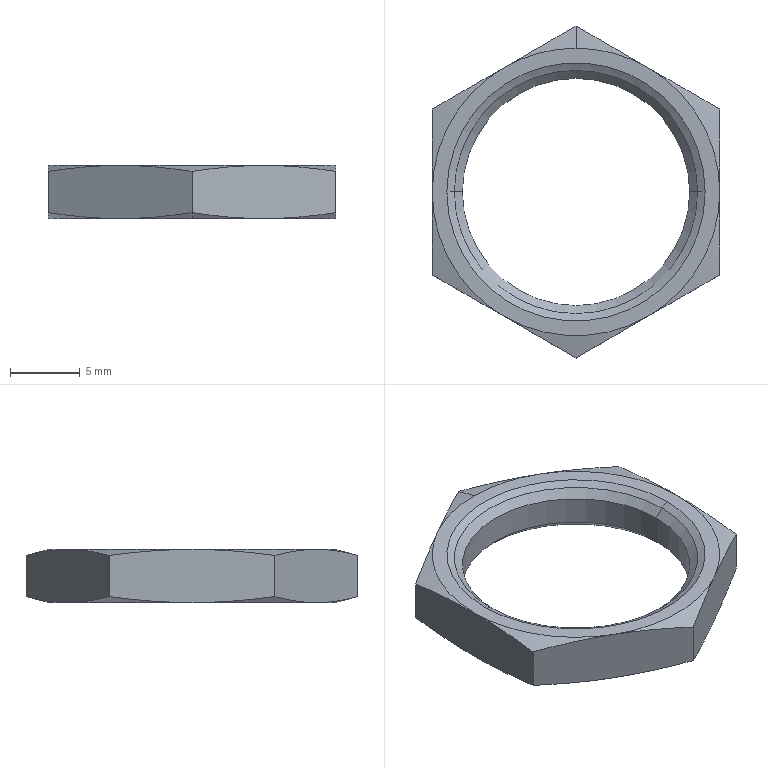Part | SolidWorks | features BaseBody 1 | 1 solid | 32 faces | box 20.638 x 23.83 x 3.81 mm | volume 553.998 mm3 | cone 22 | plane 8 | cylinder 2 | commonest cylinder face diameters 16.317 x2
STEP:
#1=CARTESIAN_POINT('',(8.158,0.,-0.8871));
#2=VERTEX_POINT('',#1);
#3=CARTESIAN_POINT('',(-8.158,0.,-0.8871));
#4=VERTEX_POINT('',#3);
#5=CARTESIAN_POINT('',(0.,0.,-0.8871));
#6=DIRECTION('',(0.,0.,-1.));
#7=DIRECTION('',(-1.,0.,0.));
#8=AXIS2_PLACEMENT_3D('',#5,#6,#7);
#9=CIRCLE('',#8,8.158);
#10=EDGE_CURVE('',#2,#4,#9,.T.);
#11=ORIENTED_EDGE('',*,*,#10,.F.);
#12=CARTESIAN_POINT('',(8.158,0.,-2.923));
#13=VERTEX_POINT('',#12);
#14=CARTESIAN_POINT('',(8.158,0.,-3.81));
#15=DIRECTION('',(0.,0.,-1.));
#16=VECTOR('',#15,1000.);
#17=LINE('',#14,#16);
#18=EDGE_CURVE('',#2,#13,#17,.T.);
#19=ORIENTED_EDGE('',*,*,#18,.T.);
#20=CARTESIAN_POINT('',(-8.158,0.,-2.923));
#21=VERTEX_POINT('',#20);
#22=CARTESIAN_POINT('',(0.,0.,-2.923));
#23=DIRECTION('',(0.,0.,1.));
#24=DIRECTION('',(-1.,0.,0.));
#25=AXIS2_PLACEMENT_3D('',#22,#23,#24);
#26=CIRCLE('',#25,8.158);
#27=EDGE_CURVE('',#21,#13,#26,.T.);
#28=ORIENTED_EDGE('',*,*,#27,.F.);
#29=CARTESIAN_POINT('',(-8.158,0.,-3.81));
#30=DIRECTION('',(0.,0.,-1.));
#31=VECTOR('',#30,1000.);
#32=LINE('',#29,#31);
#33=EDGE_CURVE('',#4,#21,#32,.T.);
#34=ORIENTED_EDGE('',*,*,#33,.F.);
#35=EDGE_LOOP('',(#11,#19,#28,#34));
#36=FACE_OUTER_BOUND('',#35,.T.);
#37=CARTESIAN_POINT('',(0.,0.,-3.81));
#38=DIRECTION('',(0.,0.,-1.));
#39=DIRECTION('',(-1.,0.,0.));
#40=AXIS2_PLACEMENT_3D('',#37,#38,#39);
#41=CYLINDRICAL_SURFACE('',#40,8.158);
#42=ADVANCED_FACE('',(#36),#41,.F.);
#43=ORIENTED_EDGE('',*,*,#10,.T.);
#44=CARTESIAN_POINT('',(-8.738,0.,-0.308));
#45=VERTEX_POINT('',#44);
#46=CARTESIAN_POINT('',(-8.738,0.,-0.308));
#47=DIRECTION('',(-0.7071,0.,0.7071));
#48=VECTOR('',#47,1000.);
#49=LINE('',#46,#48);
#50=EDGE_CURVE('',#4,#45,#49,.T.);
#51=ORIENTED_EDGE('',*,*,#50,.T.);
#52=CARTESIAN_POINT('',(8.738,0.,-0.308));
#53=VERTEX_POINT('',#52);
#54=CARTESIAN_POINT('',(0.,0.,-0.308));
#55=DIRECTION('',(0.,0.,-1.));
#56=DIRECTION('',(1.,0.,0.));
#57=AXIS2_PLACEMENT_3D('',#54,#55,#56);
#58=CIRCLE('',#57,8.738);
#59=EDGE_CURVE('',#53,#45,#58,.T.);
#60=ORIENTED_EDGE('',*,*,#59,.F.);
#61=CARTESIAN_POINT('',(8.738,0.,-0.308));
#62=DIRECTION('',(0.7071,0.,0.7071));
#63=VECTOR('',#62,1000.);
#64=LINE('',#61,#63);
#65=EDGE_CURVE('',#2,#53,#64,.T.);
#66=ORIENTED_EDGE('',*,*,#65,.F.);
#67=EDGE_LOOP('',(#43,#51,#60,#66));
#68=FACE_OUTER_BOUND('',#67,.T.);
#69=CARTESIAN_POINT('',(0.,0.,-0.308));
#70=DIRECTION('',(0.,0.,1.));
#71=DIRECTION('',(1.,0.,0.));
#72=AXIS2_PLACEMENT_3D('',#69,#70,#71);
#73=CONICAL_SURFACE('',#72,8.738,0.7854);
#74=ADVANCED_FACE('',(#68),#73,.F.);
#75=ORIENTED_EDGE('',*,*,#27,.T.);
#76=CARTESIAN_POINT('',(8.738,0.,-3.502));
#77=VERTEX_POINT('',#76);
#78=CARTESIAN_POINT('',(8.738,0.,-3.502));
#79=DIRECTION('',(0.7071,0.,-0.7071));
#80=VECTOR('',#79,1000.);
#81=LINE('',#78,#80);
#82=EDGE_CURVE('',#13,#77,#81,.T.);
#83=ORIENTED_EDGE('',*,*,#82,.T.);
#84=CARTESIAN_POINT('',(0.,-8.738,-3.502));
#85=VERTEX_POINT('',#84);
#86=CARTESIAN_POINT('',(0.,0.,-3.502));
#87=DIRECTION('',(0.,0.,1.));
#88=DIRECTION('',(-1.,0.,0.));
#89=AXIS2_PLACEMENT_3D('',#86,#87,#88);
#90=CIRCLE('',#89,8.738);
#91=EDGE_CURVE('',#85,#77,#90,.T.);
#92=ORIENTED_EDGE('',*,*,#91,.F.);
#93=CARTESIAN_POINT('',(-8.738,0.,-3.502));
#94=VERTEX_POINT('',#93);
#95=CARTESIAN_POINT('',(0.,0.,-3.502));
#96=DIRECTION('',(0.,0.,1.));
#97=DIRECTION('',(-1.,0.,0.));
#98=AXIS2_PLACEMENT_3D('',#95,#96,#97);
#99=CIRCLE('',#98,8.738);
#100=EDGE_CURVE('',#94,#85,#99,.T.);
#101=ORIENTED_EDGE('',*,*,#100,.F.);
#102=CARTESIAN_POINT('',(-8.738,0.,-3.502));
#103=DIRECTION('',(-0.7071,0.,-0.7071));
#104=VECTOR('',#103,1000.);
#105=LINE('',#102,#104);
#106=EDGE_CURVE('',#21,#94,#105,.T.);
#107=ORIENTED_EDGE('',*,*,#106,.F.);
#108=EDGE_LOOP('',(#75,#83,#92,#101,#107));
#109=FACE_OUTER_BOUND('',#108,.T.);
#110=CARTESIAN_POINT('',(0.,0.,-3.502));
#111=DIRECTION('',(0.,0.,-1.));
#112=DIRECTION('',(-1.,0.,0.));
#113=AXIS2_PLACEMENT_3D('',#110,#111,#112);
#114=CONICAL_SURFACE('',#113,8.738,0.7854);
#115=ADVANCED_FACE('',(#109),#114,.F.);
#116=ORIENTED_EDGE('',*,*,#59,.T.);
#117=CARTESIAN_POINT('',(-9.271,0.,0.));
#118=VERTEX_POINT('',#117);
#119=CARTESIAN_POINT('',(-9.271,0.,0.));
#120=DIRECTION('',(-0.866,0.,0.5));
#121=VECTOR('',#120,1000.);
#122=LINE('',#119,#121);
#123=EDGE_CURVE('',#45,#118,#122,.T.);
#124=ORIENTED_EDGE('',*,*,#123,.T.);
#125=CARTESIAN_POINT('',(9.271,0.,0.));
#126=VERTEX_POINT('',#125);
#127=CARTESIAN_POINT('',(0.,0.,0.));
#128=DIRECTION('',(0.,0.,-1.));
#129=DIRECTION('',(1.,0.,0.));
#130=AXIS2_PLACEMENT_3D('',#127,#128,#129);
#131=CIRCLE('',#130,9.271);
#132=EDGE_CURVE('',#126,#118,#131,.T.);
#133=ORIENTED_EDGE('',*,*,#132,.F.);
#134=CARTESIAN_POINT('',(9.271,0.,0.));
#135=DIRECTION('',(0.866,0.,0.5));
#136=VECTOR('',#135,1000.);
#137=LINE('',#134,#136);
#138=EDGE_CURVE('',#53,#126,#137,.T.);
#139=ORIENTED_EDGE('',*,*,#138,.F.);
#140=EDGE_LOOP('',(#116,#124,#133,#139));
#141=FACE_OUTER_BOUND('',#140,.T.);
#142=CARTESIAN_POINT('',(0.,0.,0.));
#143=DIRECTION('',(0.,0.,1.));
#144=DIRECTION('',(1.,0.,0.));
#145=AXIS2_PLACEMENT_3D('',#142,#143,#144);
#146=CONICAL_SURFACE('',#145,9.271,1.047);
#147=ADVANCED_FACE('',(#141),#146,.F.);
#148=CARTESIAN_POINT('',(0.,8.738,-3.502));
#149=VERTEX_POINT('',#148);
#150=CARTESIAN_POINT('',(0.,0.,-3.502));
#151=DIRECTION('',(0.,0.,1.));
#152=DIRECTION('',(-1.,0.,0.));
#153=AXIS2_PLACEMENT_3D('',#150,#151,#152);
#154=CIRCLE('',#153,8.738);
#155=EDGE_CURVE('',#149,#94,#154,.T.);
#156=ORIENTED_EDGE('',*,*,#155,.T.);
#157=ORIENTED_EDGE('',*,*,#100,.T.);
#158=CARTESIAN_POINT('',(0.,-9.271,-3.81));
#159=VERTEX_POINT('',#158);
#160=CARTESIAN_POINT('',(0.,-9.271,-3.81));
#161=DIRECTION('',(0.,-0.866,-0.5));
#162=VECTOR('',#161,1000.);
#163=LINE('',#160,#162);
#164=EDGE_CURVE('',#85,#159,#163,.T.);
#165=ORIENTED_EDGE('',*,*,#164,.T.);
#166=CARTESIAN_POINT('',(0.,9.271,-3.81));
#167=VERTEX_POINT('',#166);
#168=CARTESIAN_POINT('',(0.,0.,-3.81));
#169=DIRECTION('',(0.,0.,1.));
#170=DIRECTION('',(0.,1.,0.));
#171=AXIS2_PLACEMENT_3D('',#168,#169,#170);
#172=CIRCLE('',#171,9.271);
#173=EDGE_CURVE('',#167,#159,#172,.T.);
#174=ORIENTED_EDGE('',*,*,#173,.F.);
#175=CARTESIAN_POINT('',(0.,9.271,-3.81));
#176=DIRECTION('',(0.,0.866,-0.5));
#177=VECTOR('',#176,1000.);
#178=LINE('',#175,#177);
#179=EDGE_CURVE('',#149,#167,#178,.T.);
#180=ORIENTED_EDGE('',*,*,#179,.F.);
#181=EDGE_LOOP('',(#156,#157,#165,#174,#180));
#182=FACE_OUTER_BOUND('',#181,.T.);
#183=CARTESIAN_POINT('',(0.,0.,-3.81));
#184=DIRECTION('',(0.,0.,-1.));
#185=DIRECTION('',(0.,1.,0.));
#186=AXIS2_PLACEMENT_3D('',#183,#184,#185);
#187=CONICAL_SURFACE('',#186,9.271,1.047);
#188=ADVANCED_FACE('',(#182),#187,.F.);
#189=CARTESIAN_POINT('',(-5.159,8.936,0.));
#190=VERTEX_POINT('',#189);
#191=CARTESIAN_POINT('',(0.,10.319,0.));
#192=VERTEX_POINT('',#191);
#193=CARTESIAN_POINT('',(0.,0.,0.));
#194=DIRECTION('',(0.,0.,-1.));
#195=DIRECTION('',(0.,1.,0.));
#196=AXIS2_PLACEMENT_3D('',#193,#194,#195);
#197=CIRCLE('',#196,10.319);
#198=EDGE_CURVE('',#190,#192,#197,.T.);
#199=ORIENTED_EDGE('',*,*,#198,.T.);
#200=CARTESIAN_POINT('',(0.000000011,11.915,-0.4277));
#201=VERTEX_POINT('',#200);
#202=CARTESIAN_POINT('',(0.,11.925,-0.4303));
#203=DIRECTION('',(0.,0.9659,-0.2588));
#204=VECTOR('',#203,1000.);
#205=LINE('',#202,#204);
#206=EDGE_CURVE('',#192,#201,#205,.T.);
#207=ORIENTED_EDGE('',*,*,#206,.T.);
#208=CARTESIAN_POINT('',(0.000000011,11.915,-0.4277));
#209=CARTESIAN_POINT('',(-0.8561,11.421,-0.2953));
#210=CARTESIAN_POINT('',(-1.714,10.926,-0.1874));
#211=CARTESIAN_POINT('',(-3.433,9.933,-0.0395));
#212=CARTESIAN_POINT('',(-4.295,9.435,0.));
#213=CARTESIAN_POINT('',(-5.159,8.936,0.));
#214=B_SPLINE_CURVE_WITH_KNOTS('',3,(#208,#209,#210,#211,#212,#213),.UNSPECIFIED.,.F.,.F.,(4,2,4),(0.,0.002986,0.005973),.UNSPECIFIED.);
#215=EDGE_CURVE('',#201,#190,#214,.T.);
#216=ORIENTED_EDGE('',*,*,#215,.T.);
#217=EDGE_LOOP('',(#199,#207,#216));
#218=FACE_OUTER_BOUND('',#217,.T.);
#219=CARTESIAN_POINT('',(0.,0.,-0.4303));
#220=DIRECTION('',(0.,0.,-1.));
#221=DIRECTION('',(0.,1.,0.));
#222=AXIS2_PLACEMENT_3D('',#219,#220,#221);
#223=CONICAL_SURFACE('',#222,11.925,1.309);
#224=ADVANCED_FACE('',(#218),#223,.T.);
#225=CARTESIAN_POINT('',(-5.159,-8.936,-3.81));
#226=VERTEX_POINT('',#225);
#227=CARTESIAN_POINT('',(0.,-10.319,-3.81));
#228=VERTEX_POINT('',#227);
#229=CARTESIAN_POINT('',(0.,0.,-3.81));
#230=DIRECTION('',(0.,0.,1.));
#231=DIRECTION('',(0.,-1.,0.));
#232=AXIS2_PLACEMENT_3D('',#229,#230,#231);
#233=CIRCLE('',#232,10.319);
#234=EDGE_CURVE('',#226,#228,#233,.T.);
#235=ORIENTED_EDGE('',*,*,#234,.T.);
#236=CARTESIAN_POINT('',(0.000000011,-11.915,-3.382));
#237=VERTEX_POINT('',#236);
#238=CARTESIAN_POINT('',(0.,-11.925,-3.38));
#239=DIRECTION('',(0.,-0.9659,0.2588));
#240=VECTOR('',#239,1000.);
#241=LINE('',#238,#240);
#242=EDGE_CURVE('',#228,#237,#241,.T.);
#243=ORIENTED_EDGE('',*,*,#242,.T.);
#244=CARTESIAN_POINT('',(0.000000011,-11.915,-3.382));
#245=CARTESIAN_POINT('',(-0.8561,-11.421,-3.515));
#246=CARTESIAN_POINT('',(-1.714,-10.926,-3.623));
#247=CARTESIAN_POINT('',(-3.433,-9.933,-3.771));
#248=CARTESIAN_POINT('',(-4.295,-9.435,-3.81));
#249=CARTESIAN_POINT('',(-5.159,-8.936,-3.81));
#250=B_SPLINE_CURVE_WITH_KNOTS('',3,(#244,#245,#246,#247,#248,#249),.UNSPECIFIED.,.F.,.F.,(4,2,4),(0.,0.002986,0.005973),.UNSPECIFIED.);
#251=EDGE_CURVE('',#237,#226,#250,.T.);
#252=ORIENTED_EDGE('',*,*,#251,.T.);
#253=EDGE_LOOP('',(#235,#243,#252));
#254=FACE_OUTER_BOUND('',#253,.T.);
#255=CARTESIAN_POINT('',(0.,0.,-3.38));
#256=DIRECTION('',(0.,0.,1.));
#257=DIRECTION('',(0.,-1.,0.));
#258=AXIS2_PLACEMENT_3D('',#255,#256,#257);
#259=CONICAL_SURFACE('',#258,11.925,1.309);
#260=ADVANCED_FACE('',(#254),#259,.T.);
#261=ORIENTED_EDGE('',*,*,#18,.F.);
#262=CARTESIAN_POINT('',(0.,0.,-0.8871));
#263=DIRECTION('',(0.,0.,-1.));
#264=DIRECTION('',(-1.,0.,0.));
#265=AXIS2_PLACEMENT_3D('',#262,#263,#264);
#266=CIRCLE('',#265,8.158);
#267=EDGE_CURVE('',#4,#2,#266,.T.);
#268=ORIENTED_EDGE('',*,*,#267,.F.);
#269=ORIENTED_EDGE('',*,*,#33,.T.);
#270=CARTESIAN_POINT('',(0.,0.,-2.923));
#271=DIRECTION('',(0.,0.,1.));
#272=DIRECTION('',(-1.,0.,0.));
#273=AXIS2_PLACEMENT_3D('',#270,#271,#272);
#274=CIRCLE('',#273,8.158);
#275=EDGE_CURVE('',#13,#21,#274,.T.);
#276=ORIENTED_EDGE('',*,*,#275,.F.);
#277=EDGE_LOOP('',(#261,#268,#269,#276));
#278=FACE_OUTER_BOUND('',#277,.T.);
#279=CARTESIAN_POINT('',(0.,0.,-3.81));
#280=DIRECTION('',(0.,0.,-1.));
#281=DIRECTION('',(-1.,0.,0.));
#282=AXIS2_PLACEMENT_3D('',#279,#280,#281);
#283=CYLINDRICAL_SURFACE('',#282,8.158);
#284=ADVANCED_FACE('',(#278),#283,.F.);
#285=ORIENTED_EDGE('',*,*,#50,.F.);
#286=ORIENTED_EDGE('',*,*,#267,.T.);
#287=ORIENTED_EDGE('',*,*,#65,.T.);
#288=CARTESIAN_POINT('',(0.,0.,-0.308));
#289=DIRECTION('',(0.,0.,-1.));
#290=DIRECTION('',(1.,0.,0.));
#291=AXIS2_PLACEMENT_3D('',#288,#289,#290);
#292=CIRCLE('',#291,8.738);
#293=EDGE_CURVE('',#45,#53,#292,.T.);
#294=ORIENTED_EDGE('',*,*,#293,.F.);
#295=EDGE_LOOP('',(#285,#286,#287,#294));
#296=FACE_OUTER_BOUND('',#295,.T.);
#297=CARTESIAN_POINT('',(0.,0.,-0.308));
#298=DIRECTION('',(0.,0.,1.));
#299=DIRECTION('',(1.,0.,0.));
#300=AXIS2_PLACEMENT_3D('',#297,#298,#299);
#301=CONICAL_SURFACE('',#300,8.738,0.7854);
#302=ADVANCED_FACE('',(#296),#301,.F.);
#303=ORIENTED_EDGE('',*,*,#82,.F.);
#304=ORIENTED_EDGE('',*,*,#275,.T.);
#305=ORIENTED_EDGE('',*,*,#106,.T.);
#306=ORIENTED_EDGE('',*,*,#155,.F.);
#307=CARTESIAN_POINT('',(0.,0.,-3.502));
#308=DIRECTION('',(0.,0.,1.));
#309=DIRECTION('',(-1.,0.,0.));
#310=AXIS2_PLACEMENT_3D('',#307,#308,#309);
#311=CIRCLE('',#310,8.738);
#312=EDGE_CURVE('',#77,#149,#311,.T.);
#313=ORIENTED_EDGE('',*,*,#312,.F.);
#314=EDGE_LOOP('',(#303,#304,#305,#306,#313));
#315=FACE_OUTER_BOUND('',#314,.T.);
#316=CARTESIAN_POINT('',(0.,0.,-3.502));
#317=DIRECTION('',(0.,0.,-1.));
#318=DIRECTION('',(-1.,0.,0.));
#319=AXIS2_PLACEMENT_3D('',#316,#317,#318);
#320=CONICAL_SURFACE('',#319,8.738,0.7854);
#321=ADVANCED_FACE('',(#315),#320,.F.);
#322=ORIENTED_EDGE('',*,*,#123,.F.);
#323=ORIENTED_EDGE('',*,*,#293,.T.);
#324=ORIENTED_EDGE('',*,*,#138,.T.);
#325=CARTESIAN_POINT('',(0.,0.,0.));
#326=DIRECTION('',(0.,0.,-1.));
#327=DIRECTION('',(1.,0.,0.));
#328=AXIS2_PLACEMENT_3D('',#325,#326,#327);
#329=CIRCLE('',#328,9.271);
#330=EDGE_CURVE('',#118,#126,#329,.T.);
#331=ORIENTED_EDGE('',*,*,#330,.F.);
#332=EDGE_LOOP('',(#322,#323,#324,#331));
#333=FACE_OUTER_BOUND('',#332,.T.);
#334=CARTESIAN_POINT('',(0.,0.,0.));
#335=DIRECTION('',(0.,0.,1.));
#336=DIRECTION('',(1.,0.,0.));
#337=AXIS2_PLACEMENT_3D('',#334,#335,#336);
#338=CONICAL_SURFACE('',#337,9.271,1.047);
#339=ADVANCED_FACE('',(#333),#338,.F.);
#340=ORIENTED_EDGE('',*,*,#164,.F.);
#341=ORIENTED_EDGE('',*,*,#91,.T.);
#342=ORIENTED_EDGE('',*,*,#312,.T.);
#343=ORIENTED_EDGE('',*,*,#179,.T.);
#344=CARTESIAN_POINT('',(0.,0.,-3.81));
#345=DIRECTION('',(0.,0.,1.));
#346=DIRECTION('',(0.,1.,0.));
#347=AXIS2_PLACEMENT_3D('',#344,#345,#346);
#348=CIRCLE('',#347,9.271);
#349=EDGE_CURVE('',#159,#167,#348,.T.);
#350=ORIENTED_EDGE('',*,*,#349,.F.);
#351=EDGE_LOOP('',(#340,#341,#342,#343,#350));
#352=FACE_OUTER_BOUND('',#351,.T.);
#353=CARTESIAN_POINT('',(0.,0.,-3.81));
#354=DIRECTION('',(0.,0.,-1.));
#355=DIRECTION('',(0.,1.,0.));
#356=AXIS2_PLACEMENT_3D('',#353,#354,#355);
#357=CONICAL_SURFACE('',#356,9.271,1.047);
#358=ADVANCED_FACE('',(#352),#357,.F.);
#359=ORIENTED_EDGE('',*,*,#132,.T.);
#360=ORIENTED_EDGE('',*,*,#330,.T.);
#361=EDGE_LOOP('',(#359,#360));
#362=FACE_BOUND('',#361,.T.);
#363=CARTESIAN_POINT('',(-10.319,0.,0.));
#364=VERTEX_POINT('',#363);
#365=CARTESIAN_POINT('',(0.,0.,0.));
#366=DIRECTION('',(0.,0.,-1.));
#367=DIRECTION('',(-1.,0.,0.));
#368=AXIS2_PLACEMENT_3D('',#365,#366,#367);
#369=CIRCLE('',#368,10.319);
#370=EDGE_CURVE('',#364,#190,#369,.T.);
#371=ORIENTED_EDGE('',*,*,#370,.F.);
#372=CARTESIAN_POINT('',(-5.159,-8.936,0.));
#373=VERTEX_POINT('',#372);
#374=CARTESIAN_POINT('',(0.,0.,0.));
#375=DIRECTION('',(0.,0.,-1.));
#376=DIRECTION('',(-1.,0.,0.));
#377=AXIS2_PLACEMENT_3D('',#374,#375,#376);
#378=CIRCLE('',#377,10.319);
#379=EDGE_CURVE('',#373,#364,#378,.T.);
#380=ORIENTED_EDGE('',*,*,#379,.F.);
#381=CARTESIAN_POINT('',(5.159,-8.936,0.));
#382=VERTEX_POINT('',#381);
#383=CARTESIAN_POINT('',(0.,0.,0.));
#384=DIRECTION('',(0.,0.,-1.));
#385=DIRECTION('',(0.,1.,0.));
#386=AXIS2_PLACEMENT_3D('',#383,#384,#385);
#387=CIRCLE('',#386,10.319);
#388=EDGE_CURVE('',#382,#373,#387,.T.);
#389=ORIENTED_EDGE('',*,*,#388,.F.);
#390=CARTESIAN_POINT('',(10.319,0.,0.));
#391=VERTEX_POINT('',#390);
#392=CARTESIAN_POINT('',(0.,0.,0.));
#393=DIRECTION('',(0.,0.,-1.));
#394=DIRECTION('',(-1.,0.,0.));
#395=AXIS2_PLACEMENT_3D('',#392,#393,#394);
#396=CIRCLE('',#395,10.319);
#397=EDGE_CURVE('',#391,#382,#396,.T.);
#398=ORIENTED_EDGE('',*,*,#397,.F.);
#399=CARTESIAN_POINT('',(5.159,8.936,0.));
#400=VERTEX_POINT('',#399);
#401=CARTESIAN_POINT('',(0.,0.,0.));
#402=DIRECTION('',(0.,0.,-1.));
#403=DIRECTION('',(-1.,0.,0.));
#404=AXIS2_PLACEMENT_3D('',#401,#402,#403);
#405=CIRCLE('',#404,10.319);
#406=EDGE_CURVE('',#400,#391,#405,.T.);
#407=ORIENTED_EDGE('',*,*,#406,.F.);
#408=CARTESIAN_POINT('',(0.,0.,0.));
#409=DIRECTION('',(0.,0.,-1.));
#410=DIRECTION('',(0.,1.,0.));
#411=AXIS2_PLACEMENT_3D('',#408,#409,#410);
#412=CIRCLE('',#411,10.319);
#413=EDGE_CURVE('',#192,#400,#412,.T.);
#414=ORIENTED_EDGE('',*,*,#413,.F.);
#415=ORIENTED_EDGE('',*,*,#198,.F.);
#416=EDGE_LOOP('',(#371,#380,#389,#398,#407,#414,#415));
#417=FACE_OUTER_BOUND('',#416,.T.);
#418=CARTESIAN_POINT('',(0.,0.,0.));
#419=DIRECTION('',(0.,0.,-1.));
#420=DIRECTION('',(-1.,0.,0.));
#421=AXIS2_PLACEMENT_3D('',#418,#419,#420);
#422=PLANE('',#421);
#423=ADVANCED_FACE('',(#362,#417),#422,.F.);
#424=CARTESIAN_POINT('',(5.159,8.936,-3.81));
#425=VERTEX_POINT('',#424);
#426=CARTESIAN_POINT('',(-5.159,8.936,-3.81));
#427=VERTEX_POINT('',#426);
#428=CARTESIAN_POINT('',(0.,0.,-3.81));
#429=DIRECTION('',(0.,0.,1.));
#430=DIRECTION('',(0.,-1.,0.));
#431=AXIS2_PLACEMENT_3D('',#428,#429,#430);
#432=CIRCLE('',#431,10.319);
#433=EDGE_CURVE('',#425,#427,#432,.T.);
#434=ORIENTED_EDGE('',*,*,#433,.F.);
#435=CARTESIAN_POINT('',(10.319,0.,-3.81));
#436=VERTEX_POINT('',#435);
#437=CARTESIAN_POINT('',(0.,0.,-3.81));
#438=DIRECTION('',(0.,0.,1.));
#439=DIRECTION('',(1.,0.,0.));
#440=AXIS2_PLACEMENT_3D('',#437,#438,#439);
#441=CIRCLE('',#440,10.319);
#442=EDGE_CURVE('',#436,#425,#441,.T.);
#443=ORIENTED_EDGE('',*,*,#442,.F.);
#444=CARTESIAN_POINT('',(5.159,-8.936,-3.81));
#445=VERTEX_POINT('',#444);
#446=CARTESIAN_POINT('',(0.,0.,-3.81));
#447=DIRECTION('',(0.,0.,1.));
#448=DIRECTION('',(1.,0.,0.));
#449=AXIS2_PLACEMENT_3D('',#446,#447,#448);
#450=CIRCLE('',#449,10.319);
#451=EDGE_CURVE('',#445,#436,#450,.T.);
#452=ORIENTED_EDGE('',*,*,#451,.F.);
#453=CARTESIAN_POINT('',(0.,0.,-3.81));
#454=DIRECTION('',(0.,0.,1.));
#455=DIRECTION('',(0.,-1.,0.));
#456=AXIS2_PLACEMENT_3D('',#453,#454,#455);
#457=CIRCLE('',#456,10.319);
#458=EDGE_CURVE('',#228,#445,#457,.T.);
#459=ORIENTED_EDGE('',*,*,#458,.F.);
#460=ORIENTED_EDGE('',*,*,#234,.F.);
#461=CARTESIAN_POINT('',(-10.319,0.,-3.81));
#462=VERTEX_POINT('',#461);
#463=CARTESIAN_POINT('',(0.,0.,-3.81));
#464=DIRECTION('',(0.,0.,1.));
#465=DIRECTION('',(1.,0.,0.));
#466=AXIS2_PLACEMENT_3D('',#463,#464,#465);
#467=CIRCLE('',#466,10.319);
#468=EDGE_CURVE('',#462,#226,#467,.T.);
#469=ORIENTED_EDGE('',*,*,#468,.F.);
#470=CARTESIAN_POINT('',(0.,0.,-3.81));
#471=DIRECTION('',(0.,0.,1.));
#472=DIRECTION('',(1.,0.,0.));
#473=AXIS2_PLACEMENT_3D('',#470,#471,#472);
#474=CIRCLE('',#473,10.319);
#475=EDGE_CURVE('',#427,#462,#474,.T.);
#476=ORIENTED_EDGE('',*,*,#475,.F.);
#477=EDGE_LOOP('',(#434,#443,#452,#459,#460,#469,#476));
#478=FACE_OUTER_BOUND('',#477,.T.);
#479=ORIENTED_EDGE('',*,*,#173,.T.);
#480=ORIENTED_EDGE('',*,*,#349,.T.);
#481=EDGE_LOOP('',(#479,#480));
#482=FACE_BOUND('',#481,.T.);
#483=CARTESIAN_POINT('',(0.,10.319,-3.81));
#484=DIRECTION('',(0.,0.,1.));
#485=DIRECTION('',(1.,0.,0.));
#486=AXIS2_PLACEMENT_3D('',#483,#484,#485);
#487=PLANE('',#486);
#488=ADVANCED_FACE('',(#478,#482),#487,.F.);
#489=ORIENTED_EDGE('',*,*,#206,.F.);
#490=ORIENTED_EDGE('',*,*,#413,.T.);
#491=CARTESIAN_POINT('',(5.159,8.936,0.));
#492=CARTESIAN_POINT('',(4.295,9.435,0.));
#493=CARTESIAN_POINT('',(3.433,9.933,-0.0395));
#494=CARTESIAN_POINT('',(1.714,10.926,-0.1874));
#495=CARTESIAN_POINT('',(0.8561,11.421,-0.2953));
#496=CARTESIAN_POINT('',(0.000000011,11.915,-0.4277));
#497=B_SPLINE_CURVE_WITH_KNOTS('',3,(#491,#492,#493,#494,#495,#496),.UNSPECIFIED.,.F.,.F.,(4,2,4),(0.,0.002986,0.005973),.UNSPECIFIED.);
#498=EDGE_CURVE('',#400,#201,#497,.T.);
#499=ORIENTED_EDGE('',*,*,#498,.T.);
#500=EDGE_LOOP('',(#489,#490,#499));
#501=FACE_OUTER_BOUND('',#500,.T.);
#502=CARTESIAN_POINT('',(0.,0.,-0.4303));
#503=DIRECTION('',(0.,0.,-1.));
#504=DIRECTION('',(0.,1.,0.));
#505=AXIS2_PLACEMENT_3D('',#502,#503,#504);
#506=CONICAL_SURFACE('',#505,11.925,1.309);
#507=ADVANCED_FACE('',(#501),#506,.T.);
#508=ORIENTED_EDGE('',*,*,#370,.T.);
#509=CARTESIAN_POINT('',(-10.319,5.958,-0.4277));
#510=VERTEX_POINT('',#509);
#511=CARTESIAN_POINT('',(-5.159,8.936,0.));
#512=CARTESIAN_POINT('',(-6.024,8.437,0.));
#513=CARTESIAN_POINT('',(-6.886,7.94,-0.0395));
#514=CARTESIAN_POINT('',(-8.605,6.947,-0.1874));
#515=CARTESIAN_POINT('',(-9.463,6.452,-0.2953));
#516=CARTESIAN_POINT('',(-10.319,5.958,-0.4277));
#517=B_SPLINE_CURVE_WITH_KNOTS('',3,(#511,#512,#513,#514,#515,#516),.UNSPECIFIED.,.F.,.F.,(4,2,4),(0.,0.002986,0.005973),.UNSPECIFIED.);
#518=EDGE_CURVE('',#190,#510,#517,.T.);
#519=ORIENTED_EDGE('',*,*,#518,.T.);
#520=CARTESIAN_POINT('',(-10.319,5.958,-0.4277));
#521=CARTESIAN_POINT('',(-10.319,4.969,-0.2953));
#522=CARTESIAN_POINT('',(-10.319,3.979,-0.1874));
#523=CARTESIAN_POINT('',(-10.319,1.993,-0.0395));
#524=CARTESIAN_POINT('',(-10.319,0.998,0.));
#525=CARTESIAN_POINT('',(-10.319,0.,0.));
#526=B_SPLINE_CURVE_WITH_KNOTS('',3,(#520,#521,#522,#523,#524,#525),.UNSPECIFIED.,.F.,.F.,(4,2,4),(0.,0.002986,0.005973),.UNSPECIFIED.);
#527=EDGE_CURVE('',#510,#364,#526,.T.);
#528=ORIENTED_EDGE('',*,*,#527,.T.);
#529=EDGE_LOOP('',(#508,#519,#528));
#530=FACE_OUTER_BOUND('',#529,.T.);
#531=CARTESIAN_POINT('',(0.,0.,-0.4303));
#532=DIRECTION('',(0.,0.,-1.));
#533=DIRECTION('',(-1.,0.,0.));
#534=AXIS2_PLACEMENT_3D('',#531,#532,#533);
#535=CONICAL_SURFACE('',#534,11.925,1.309);
#536=ADVANCED_FACE('',(#530),#535,.T.);
#537=CARTESIAN_POINT('',(-10.319,-5.958,-0.4277));
#538=VERTEX_POINT('',#537);
#539=CARTESIAN_POINT('',(-10.319,-5.958,-0.4277));
#540=CARTESIAN_POINT('',(-9.463,-6.452,-0.2953));
#541=CARTESIAN_POINT('',(-8.605,-6.947,-0.1874));
#542=CARTESIAN_POINT('',(-6.886,-7.94,-0.0395));
#543=CARTESIAN_POINT('',(-6.024,-8.437,0.));
#544=CARTESIAN_POINT('',(-5.159,-8.936,0.));
#545=B_SPLINE_CURVE_WITH_KNOTS('',3,(#539,#540,#541,#542,#543,#544),.UNSPECIFIED.,.F.,.F.,(4,2,4),(0.,0.002986,0.005973),.UNSPECIFIED.);
#546=EDGE_CURVE('',#538,#373,#545,.T.);
#547=ORIENTED_EDGE('',*,*,#546,.T.);
#548=ORIENTED_EDGE('',*,*,#379,.T.);
#549=CARTESIAN_POINT('',(-10.319,0.,0.));
#550=CARTESIAN_POINT('',(-10.319,-0.998,0.));
#551=CARTESIAN_POINT('',(-10.319,-1.993,-0.0395));
#552=CARTESIAN_POINT('',(-10.319,-3.979,-0.1874));
#553=CARTESIAN_POINT('',(-10.319,-4.969,-0.2953));
#554=CARTESIAN_POINT('',(-10.319,-5.958,-0.4277));
#555=B_SPLINE_CURVE_WITH_KNOTS('',3,(#549,#550,#551,#552,#553,#554),.UNSPECIFIED.,.F.,.F.,(4,2,4),(0.,0.002986,0.005973),.UNSPECIFIED.);
#556=EDGE_CURVE('',#364,#538,#555,.T.);
#557=ORIENTED_EDGE('',*,*,#556,.T.);
#558=EDGE_LOOP('',(#547,#548,#557));
#559=FACE_OUTER_BOUND('',#558,.T.);
#560=CARTESIAN_POINT('',(0.,0.,-0.4303));
#561=DIRECTION('',(0.,0.,-1.));
#562=DIRECTION('',(-1.,0.,0.));
#563=AXIS2_PLACEMENT_3D('',#560,#561,#562);
#564=CONICAL_SURFACE('',#563,11.925,1.309);
#565=ADVANCED_FACE('',(#559),#564,.T.);
#566=ORIENTED_EDGE('',*,*,#388,.T.);
#567=CARTESIAN_POINT('',(0.00000002,-11.915,-0.4277));
#568=VERTEX_POINT('',#567);
#569=CARTESIAN_POINT('',(-5.159,-8.936,0.));
#570=CARTESIAN_POINT('',(-4.295,-9.435,0.));
#571=CARTESIAN_POINT('',(-3.433,-9.933,-0.0395));
#572=CARTESIAN_POINT('',(-1.714,-10.926,-0.1874));
#573=CARTESIAN_POINT('',(-0.8561,-11.421,-0.2953));
#574=CARTESIAN_POINT('',(0.00000002,-11.915,-0.4277));
#575=B_SPLINE_CURVE_WITH_KNOTS('',3,(#569,#570,#571,#572,#573,#574),.UNSPECIFIED.,.F.,.F.,(4,2,4),(0.,0.002986,0.005973),.UNSPECIFIED.);
#576=EDGE_CURVE('',#373,#568,#575,.T.);
#577=ORIENTED_EDGE('',*,*,#576,.T.);
#578=CARTESIAN_POINT('',(0.00000002,-11.915,-0.4277));
#579=CARTESIAN_POINT('',(0.8561,-11.421,-0.2953));
#580=CARTESIAN_POINT('',(1.714,-10.926,-0.1874));
#581=CARTESIAN_POINT('',(3.433,-9.933,-0.0395));
#582=CARTESIAN_POINT('',(4.295,-9.435,0.));
#583=CARTESIAN_POINT('',(5.159,-8.936,0.));
#584=B_SPLINE_CURVE_WITH_KNOTS('',3,(#578,#579,#580,#581,#582,#583),.UNSPECIFIED.,.F.,.F.,(4,2,4),(0.,0.002986,0.005973),.UNSPECIFIED.);
#585=EDGE_CURVE('',#568,#382,#584,.T.);
#586=ORIENTED_EDGE('',*,*,#585,.T.);
#587=EDGE_LOOP('',(#566,#577,#586));
#588=FACE_OUTER_BOUND('',#587,.T.);
#589=CARTESIAN_POINT('',(0.,0.,-0.4303));
#590=DIRECTION('',(0.,0.,-1.));
#591=DIRECTION('',(0.,1.,0.));
#592=AXIS2_PLACEMENT_3D('',#589,#590,#591);
#593=CONICAL_SURFACE('',#592,11.925,1.309);
#594=ADVANCED_FACE('',(#588),#593,.T.);
#595=ORIENTED_EDGE('',*,*,#397,.T.);
#596=CARTESIAN_POINT('',(10.319,-5.958,-0.4277));
#597=VERTEX_POINT('',#596);
#598=CARTESIAN_POINT('',(5.159,-8.936,0.));
#599=CARTESIAN_POINT('',(6.024,-8.437,0.));
#600=CARTESIAN_POINT('',(6.886,-7.94,-0.0395));
#601=CARTESIAN_POINT('',(8.605,-6.947,-0.1874));
#602=CARTESIAN_POINT('',(9.463,-6.452,-0.2953));
#603=CARTESIAN_POINT('',(10.319,-5.958,-0.4277));
#604=B_SPLINE_CURVE_WITH_KNOTS('',3,(#598,#599,#600,#601,#602,#603),.UNSPECIFIED.,.F.,.F.,(4,2,4),(0.,0.002986,0.005973),.UNSPECIFIED.);
#605=EDGE_CURVE('',#382,#597,#604,.T.);
#606=ORIENTED_EDGE('',*,*,#605,.T.);
#607=CARTESIAN_POINT('',(10.319,-5.958,-0.4277));
#608=CARTESIAN_POINT('',(10.319,-4.969,-0.2953));
#609=CARTESIAN_POINT('',(10.319,-3.979,-0.1874));
#610=CARTESIAN_POINT('',(10.319,-1.993,-0.0395));
#611=CARTESIAN_POINT('',(10.319,-0.998,0.));
#612=CARTESIAN_POINT('',(10.319,0.,0.));
#613=B_SPLINE_CURVE_WITH_KNOTS('',3,(#607,#608,#609,#610,#611,#612),.UNSPECIFIED.,.F.,.F.,(4,2,4),(0.,0.002986,0.005973),.UNSPECIFIED.);
#614=EDGE_CURVE('',#597,#391,#613,.T.);
#615=ORIENTED_EDGE('',*,*,#614,.T.);
#616=EDGE_LOOP('',(#595,#606,#615));
#617=FACE_OUTER_BOUND('',#616,.T.);
#618=CARTESIAN_POINT('',(0.,0.,-0.4303));
#619=DIRECTION('',(0.,0.,-1.));
#620=DIRECTION('',(-1.,0.,0.));
#621=AXIS2_PLACEMENT_3D('',#618,#619,#620);
#622=CONICAL_SURFACE('',#621,11.925,1.309);
#623=ADVANCED_FACE('',(#617),#622,.T.);
#624=ORIENTED_EDGE('',*,*,#406,.T.);
#625=CARTESIAN_POINT('',(10.319,5.958,-0.4277));
#626=VERTEX_POINT('',#625);
#627=CARTESIAN_POINT('',(10.319,0.,0.));
#628=CARTESIAN_POINT('',(10.319,0.998,0.));
#629=CARTESIAN_POINT('',(10.319,1.993,-0.0395));
#630=CARTESIAN_POINT('',(10.319,3.979,-0.1874));
#631=CARTESIAN_POINT('',(10.319,4.969,-0.2953));
#632=CARTESIAN_POINT('',(10.319,5.958,-0.4277));
#633=B_SPLINE_CURVE_WITH_KNOTS('',3,(#627,#628,#629,#630,#631,#632),.UNSPECIFIED.,.F.,.F.,(4,2,4),(0.,0.002986,0.005973),.UNSPECIFIED.);
#634=EDGE_CURVE('',#391,#626,#633,.T.);
#635=ORIENTED_EDGE('',*,*,#634,.T.);
#636=CARTESIAN_POINT('',(10.319,5.958,-0.4277));
#637=CARTESIAN_POINT('',(9.463,6.452,-0.2953));
#638=CARTESIAN_POINT('',(8.605,6.947,-0.1874));
#639=CARTESIAN_POINT('',(6.886,7.94,-0.0395));
#640=CARTESIAN_POINT('',(6.024,8.437,0.));
#641=CARTESIAN_POINT('',(5.159,8.936,0.));
#642=B_SPLINE_CURVE_WITH_KNOTS('',3,(#636,#637,#638,#639,#640,#641),.UNSPECIFIED.,.F.,.F.,(4,2,4),(0.,0.002986,0.005973),.UNSPECIFIED.);
#643=EDGE_CURVE('',#626,#400,#642,.T.);
#644=ORIENTED_EDGE('',*,*,#643,.T.);
#645=EDGE_LOOP('',(#624,#635,#644));
#646=FACE_OUTER_BOUND('',#645,.T.);
#647=CARTESIAN_POINT('',(0.,0.,-0.4303));
#648=DIRECTION('',(0.,0.,-1.));
#649=DIRECTION('',(-1.,0.,0.));
#650=AXIS2_PLACEMENT_3D('',#647,#648,#649);
#651=CONICAL_SURFACE('',#650,11.925,1.309);
#652=ADVANCED_FACE('',(#646),#651,.T.);
#653=ORIENTED_EDGE('',*,*,#475,.T.);
#654=CARTESIAN_POINT('',(-10.319,5.958,-3.382));
#655=VERTEX_POINT('',#654);
#656=CARTESIAN_POINT('',(-10.319,0.,-3.81));
#657=CARTESIAN_POINT('',(-10.319,0.998,-3.81));
#658=CARTESIAN_POINT('',(-10.319,1.993,-3.771));
#659=CARTESIAN_POINT('',(-10.319,3.979,-3.623));
#660=CARTESIAN_POINT('',(-10.319,4.969,-3.515));
#661=CARTESIAN_POINT('',(-10.319,5.958,-3.382));
#662=B_SPLINE_CURVE_WITH_KNOTS('',3,(#656,#657,#658,#659,#660,#661),.UNSPECIFIED.,.F.,.F.,(4,2,4),(0.,0.002986,0.005973),.UNSPECIFIED.);
#663=EDGE_CURVE('',#462,#655,#662,.T.);
#664=ORIENTED_EDGE('',*,*,#663,.T.);
#665=CARTESIAN_POINT('',(-10.319,5.958,-3.382));
#666=CARTESIAN_POINT('',(-9.463,6.452,-3.515));
#667=CARTESIAN_POINT('',(-8.605,6.947,-3.623));
#668=CARTESIAN_POINT('',(-6.886,7.94,-3.771));
#669=CARTESIAN_POINT('',(-6.024,8.437,-3.81));
#670=CARTESIAN_POINT('',(-5.159,8.936,-3.81));
#671=B_SPLINE_CURVE_WITH_KNOTS('',3,(#665,#666,#667,#668,#669,#670),.UNSPECIFIED.,.F.,.F.,(4,2,4),(0.,0.002986,0.005973),.UNSPECIFIED.);
#672=EDGE_CURVE('',#655,#427,#671,.T.);
#673=ORIENTED_EDGE('',*,*,#672,.T.);
#674=EDGE_LOOP('',(#653,#664,#673));
#675=FACE_OUTER_BOUND('',#674,.T.);
#676=CARTESIAN_POINT('',(0.,0.,-3.38));
#677=DIRECTION('',(0.,0.,1.));
#678=DIRECTION('',(1.,0.,0.));
#679=AXIS2_PLACEMENT_3D('',#676,#677,#678);
#680=CONICAL_SURFACE('',#679,11.925,1.309);
#681=ADVANCED_FACE('',(#675),#680,.T.);
#682=CARTESIAN_POINT('',(-0.000000042,11.915,-3.382));
#683=VERTEX_POINT('',#682);
#684=CARTESIAN_POINT('',(-0.000000042,11.915,-3.382));
#685=CARTESIAN_POINT('',(0.8561,11.421,-3.515));
#686=CARTESIAN_POINT('',(1.714,10.926,-3.623));
#687=CARTESIAN_POINT('',(3.433,9.933,-3.771));
#688=CARTESIAN_POINT('',(4.295,9.435,-3.81));
#689=CARTESIAN_POINT('',(5.159,8.936,-3.81));
#690=B_SPLINE_CURVE_WITH_KNOTS('',3,(#684,#685,#686,#687,#688,#689),.UNSPECIFIED.,.F.,.F.,(4,2,4),(0.,0.002986,0.005973),.UNSPECIFIED.);
#691=EDGE_CURVE('',#683,#425,#690,.T.);
#692=ORIENTED_EDGE('',*,*,#691,.T.);
#693=ORIENTED_EDGE('',*,*,#433,.T.);
#694=CARTESIAN_POINT('',(-5.159,8.936,-3.81));
#695=CARTESIAN_POINT('',(-4.295,9.435,-3.81));
#696=CARTESIAN_POINT('',(-3.433,9.933,-3.771));
#697=CARTESIAN_POINT('',(-1.714,10.926,-3.623));
#698=CARTESIAN_POINT('',(-0.8561,11.421,-3.515));
#699=CARTESIAN_POINT('',(-0.000000042,11.915,-3.382));
#700=B_SPLINE_CURVE_WITH_KNOTS('',3,(#694,#695,#696,#697,#698,#699),.UNSPECIFIED.,.F.,.F.,(4,2,4),(0.,0.002986,0.005973),.UNSPECIFIED.);
#701=EDGE_CURVE('',#427,#683,#700,.T.);
#702=ORIENTED_EDGE('',*,*,#701,.T.);
#703=EDGE_LOOP('',(#692,#693,#702));
#704=FACE_OUTER_BOUND('',#703,.T.);
#705=CARTESIAN_POINT('',(0.,0.,-3.38));
#706=DIRECTION('',(0.,0.,1.));
#707=DIRECTION('',(0.,-1.,0.));
#708=AXIS2_PLACEMENT_3D('',#705,#706,#707);
#709=CONICAL_SURFACE('',#708,11.925,1.309);
#710=ADVANCED_FACE('',(#704),#709,.T.);
#711=CARTESIAN_POINT('',(10.319,5.958,-3.382));
#712=VERTEX_POINT('',#711);
#713=CARTESIAN_POINT('',(10.319,5.958,-3.382));
#714=CARTESIAN_POINT('',(10.319,4.969,-3.515));
#715=CARTESIAN_POINT('',(10.319,3.979,-3.623));
#716=CARTESIAN_POINT('',(10.319,1.993,-3.771));
#717=CARTESIAN_POINT('',(10.319,0.998,-3.81));
#718=CARTESIAN_POINT('',(10.319,0.,-3.81));
#719=B_SPLINE_CURVE_WITH_KNOTS('',3,(#713,#714,#715,#716,#717,#718),.UNSPECIFIED.,.F.,.F.,(4,2,4),(0.,0.002986,0.005973),.UNSPECIFIED.);
#720=EDGE_CURVE('',#712,#436,#719,.T.);
#721=ORIENTED_EDGE('',*,*,#720,.T.);
#722=ORIENTED_EDGE('',*,*,#442,.T.);
#723=CARTESIAN_POINT('',(5.159,8.936,-3.81));
#724=CARTESIAN_POINT('',(6.024,8.437,-3.81));
#725=CARTESIAN_POINT('',(6.886,7.94,-3.771));
#726=CARTESIAN_POINT('',(8.605,6.947,-3.623));
#727=CARTESIAN_POINT('',(9.463,6.452,-3.515));
#728=CARTESIAN_POINT('',(10.319,5.958,-3.382));
#729=B_SPLINE_CURVE_WITH_KNOTS('',3,(#723,#724,#725,#726,#727,#728),.UNSPECIFIED.,.F.,.F.,(4,2,4),(0.,0.002986,0.005973),.UNSPECIFIED.);
#730=EDGE_CURVE('',#425,#712,#729,.T.);
#731=ORIENTED_EDGE('',*,*,#730,.T.);
#732=EDGE_LOOP('',(#721,#722,#731));
#733=FACE_OUTER_BOUND('',#732,.T.);
#734=CARTESIAN_POINT('',(0.,0.,-3.38));
#735=DIRECTION('',(0.,0.,1.));
#736=DIRECTION('',(1.,0.,0.));
#737=AXIS2_PLACEMENT_3D('',#734,#735,#736);
#738=CONICAL_SURFACE('',#737,11.925,1.309);
#739=ADVANCED_FACE('',(#733),#738,.T.);
#740=CARTESIAN_POINT('',(10.319,-5.958,-3.382));
#741=VERTEX_POINT('',#740);
#742=CARTESIAN_POINT('',(10.319,-5.958,-3.382));
#743=CARTESIAN_POINT('',(9.463,-6.452,-3.515));
#744=CARTESIAN_POINT('',(8.605,-6.947,-3.623));
#745=CARTESIAN_POINT('',(6.886,-7.94,-3.771));
#746=CARTESIAN_POINT('',(6.024,-8.437,-3.81));
#747=CARTESIAN_POINT('',(5.159,-8.936,-3.81));
#748=B_SPLINE_CURVE_WITH_KNOTS('',3,(#742,#743,#744,#745,#746,#747),.UNSPECIFIED.,.F.,.F.,(4,2,4),(0.,0.002986,0.005973),.UNSPECIFIED.);
#749=EDGE_CURVE('',#741,#445,#748,.T.);
#750=ORIENTED_EDGE('',*,*,#749,.T.);
#751=ORIENTED_EDGE('',*,*,#451,.T.);
#752=CARTESIAN_POINT('',(10.319,0.,-3.81));
#753=CARTESIAN_POINT('',(10.319,-0.998,-3.81));
#754=CARTESIAN_POINT('',(10.319,-1.993,-3.771));
#755=CARTESIAN_POINT('',(10.319,-3.979,-3.623));
#756=CARTESIAN_POINT('',(10.319,-4.969,-3.515));
#757=CARTESIAN_POINT('',(10.319,-5.958,-3.382));
#758=B_SPLINE_CURVE_WITH_KNOTS('',3,(#752,#753,#754,#755,#756,#757),.UNSPECIFIED.,.F.,.F.,(4,2,4),(0.,0.002986,0.005973),.UNSPECIFIED.);
#759=EDGE_CURVE('',#436,#741,#758,.T.);
#760=ORIENTED_EDGE('',*,*,#759,.T.);
#761=EDGE_LOOP('',(#750,#751,#760));
#762=FACE_OUTER_BOUND('',#761,.T.);
#763=CARTESIAN_POINT('',(0.,0.,-3.38));
#764=DIRECTION('',(0.,0.,1.));
#765=DIRECTION('',(1.,0.,0.));
#766=AXIS2_PLACEMENT_3D('',#763,#764,#765);
#767=CONICAL_SURFACE('',#766,11.925,1.309);
#768=ADVANCED_FACE('',(#762),#767,.T.);
#769=ORIENTED_EDGE('',*,*,#242,.F.);
#770=ORIENTED_EDGE('',*,*,#458,.T.);
#771=CARTESIAN_POINT('',(5.159,-8.936,-3.81));
#772=CARTESIAN_POINT('',(4.295,-9.435,-3.81));
#773=CARTESIAN_POINT('',(3.433,-9.933,-3.771));
#774=CARTESIAN_POINT('',(1.714,-10.926,-3.623));
#775=CARTESIAN_POINT('',(0.8561,-11.421,-3.515));
#776=CARTESIAN_POINT('',(0.000000011,-11.915,-3.382));
#777=B_SPLINE_CURVE_WITH_KNOTS('',3,(#771,#772,#773,#774,#775,#776),.UNSPECIFIED.,.F.,.F.,(4,2,4),(0.,0.002986,0.005973),.UNSPECIFIED.);
#778=EDGE_CURVE('',#445,#237,#777,.T.);
#779=ORIENTED_EDGE('',*,*,#778,.T.);
#780=EDGE_LOOP('',(#769,#770,#779));
#781=FACE_OUTER_BOUND('',#780,.T.);
#782=CARTESIAN_POINT('',(0.,0.,-3.38));
#783=DIRECTION('',(0.,0.,1.));
#784=DIRECTION('',(0.,-1.,0.));
#785=AXIS2_PLACEMENT_3D('',#782,#783,#784);
#786=CONICAL_SURFACE('',#785,11.925,1.309);
#787=ADVANCED_FACE('',(#781),#786,.T.);
#788=ORIENTED_EDGE('',*,*,#468,.T.);
#789=CARTESIAN_POINT('',(-10.319,-5.958,-3.382));
#790=VERTEX_POINT('',#789);
#791=CARTESIAN_POINT('',(-5.159,-8.936,-3.81));
#792=CARTESIAN_POINT('',(-6.024,-8.437,-3.81));
#793=CARTESIAN_POINT('',(-6.886,-7.94,-3.771));
#794=CARTESIAN_POINT('',(-8.605,-6.947,-3.623));
#795=CARTESIAN_POINT('',(-9.463,-6.452,-3.515));
#796=CARTESIAN_POINT('',(-10.319,-5.958,-3.382));
#797=B_SPLINE_CURVE_WITH_KNOTS('',3,(#791,#792,#793,#794,#795,#796),.UNSPECIFIED.,.F.,.F.,(4,2,4),(0.,0.002986,0.005973),.UNSPECIFIED.);
#798=EDGE_CURVE('',#226,#790,#797,.T.);
#799=ORIENTED_EDGE('',*,*,#798,.T.);
#800=CARTESIAN_POINT('',(-10.319,-5.958,-3.382));
#801=CARTESIAN_POINT('',(-10.319,-4.969,-3.515));
#802=CARTESIAN_POINT('',(-10.319,-3.979,-3.623));
#803=CARTESIAN_POINT('',(-10.319,-1.993,-3.771));
#804=CARTESIAN_POINT('',(-10.319,-0.998,-3.81));
#805=CARTESIAN_POINT('',(-10.319,0.,-3.81));
#806=B_SPLINE_CURVE_WITH_KNOTS('',3,(#800,#801,#802,#803,#804,#805),.UNSPECIFIED.,.F.,.F.,(4,2,4),(0.,0.002986,0.005973),.UNSPECIFIED.);
#807=EDGE_CURVE('',#790,#462,#806,.T.);
#808=ORIENTED_EDGE('',*,*,#807,.T.);
#809=EDGE_LOOP('',(#788,#799,#808));
#810=FACE_OUTER_BOUND('',#809,.T.);
#811=CARTESIAN_POINT('',(0.,0.,-3.38));
#812=DIRECTION('',(0.,0.,1.));
#813=DIRECTION('',(1.,0.,0.));
#814=AXIS2_PLACEMENT_3D('',#811,#812,#813);
#815=CONICAL_SURFACE('',#814,11.925,1.309);
#816=ADVANCED_FACE('',(#810),#815,.T.);
#817=ORIENTED_EDGE('',*,*,#672,.F.);
#818=CARTESIAN_POINT('',(-10.319,5.958,-3.81));
#819=DIRECTION('',(0.,0.,1.));
#820=VECTOR('',#819,1000.);
#821=LINE('',#818,#820);
#822=EDGE_CURVE('',#655,#510,#821,.T.);
#823=ORIENTED_EDGE('',*,*,#822,.T.);
#824=ORIENTED_EDGE('',*,*,#518,.F.);
#825=ORIENTED_EDGE('',*,*,#215,.F.);
#826=CARTESIAN_POINT('',(0.,11.915,-3.81));
#827=DIRECTION('',(0.,0.,-1.));
#828=VECTOR('',#827,1000.);
#829=LINE('',#826,#828);
#830=EDGE_CURVE('',#201,#683,#829,.T.);
#831=ORIENTED_EDGE('',*,*,#830,.T.);
#832=ORIENTED_EDGE('',*,*,#701,.F.);
#833=EDGE_LOOP('',(#817,#823,#824,#825,#831,#832));
#834=FACE_OUTER_BOUND('',#833,.T.);
#835=CARTESIAN_POINT('',(0.,11.915,-3.81));
#836=DIRECTION('',(-0.5,0.866,0.));
#837=DIRECTION('',(-0.866,-0.5,0.));
#838=AXIS2_PLACEMENT_3D('',#835,#836,#837);
#839=PLANE('',#838);
#840=ADVANCED_FACE('',(#834),#839,.T.);
#841=ORIENTED_EDGE('',*,*,#691,.F.);
#842=ORIENTED_EDGE('',*,*,#830,.F.);
#843=ORIENTED_EDGE('',*,*,#498,.F.);
#844=ORIENTED_EDGE('',*,*,#643,.F.);
#845=CARTESIAN_POINT('',(10.319,5.958,-3.81));
#846=DIRECTION('',(0.,0.,-1.));
#847=VECTOR('',#846,1000.);
#848=LINE('',#845,#847);
#849=EDGE_CURVE('',#626,#712,#848,.T.);
#850=ORIENTED_EDGE('',*,*,#849,.T.);
#851=ORIENTED_EDGE('',*,*,#730,.F.);
#852=EDGE_LOOP('',(#841,#842,#843,#844,#850,#851));
#853=FACE_OUTER_BOUND('',#852,.T.);
#854=CARTESIAN_POINT('',(10.319,5.958,-3.81));
#855=DIRECTION('',(0.5,0.866,0.));
#856=DIRECTION('',(-0.866,0.5,0.));
#857=AXIS2_PLACEMENT_3D('',#854,#855,#856);
#858=PLANE('',#857);
#859=ADVANCED_FACE('',(#853),#858,.T.);
#860=ORIENTED_EDGE('',*,*,#807,.F.);
#861=CARTESIAN_POINT('',(-10.319,-5.958,-3.81));
#862=DIRECTION('',(0.,0.,1.));
#863=VECTOR('',#862,1000.);
#864=LINE('',#861,#863);
#865=EDGE_CURVE('',#790,#538,#864,.T.);
#866=ORIENTED_EDGE('',*,*,#865,.T.);
#867=ORIENTED_EDGE('',*,*,#556,.F.);
#868=ORIENTED_EDGE('',*,*,#527,.F.);
#869=ORIENTED_EDGE('',*,*,#822,.F.);
#870=ORIENTED_EDGE('',*,*,#663,.F.);
#871=EDGE_LOOP('',(#860,#866,#867,#868,#869,#870));
#872=FACE_OUTER_BOUND('',#871,.T.);
#873=CARTESIAN_POINT('',(-10.319,5.958,-3.81));
#874=DIRECTION('',(-1.,0.,0.));
#875=DIRECTION('',(0.,0.,1.));
#876=AXIS2_PLACEMENT_3D('',#873,#874,#875);
#877=PLANE('',#876);
#878=ADVANCED_FACE('',(#872),#877,.T.);
#879=ORIENTED_EDGE('',*,*,#251,.F.);
#880=CARTESIAN_POINT('',(0.,-11.915,-3.81));
#881=DIRECTION('',(0.,0.,1.));
#882=VECTOR('',#881,1000.);
#883=LINE('',#880,#882);
#884=EDGE_CURVE('',#237,#568,#883,.T.);
#885=ORIENTED_EDGE('',*,*,#884,.T.);
#886=ORIENTED_EDGE('',*,*,#576,.F.);
#887=ORIENTED_EDGE('',*,*,#546,.F.);
#888=ORIENTED_EDGE('',*,*,#865,.F.);
#889=ORIENTED_EDGE('',*,*,#798,.F.);
#890=EDGE_LOOP('',(#879,#885,#886,#887,#888,#889));
#891=FACE_OUTER_BOUND('',#890,.T.);
#892=CARTESIAN_POINT('',(-10.319,-5.958,-3.81));
#893=DIRECTION('',(-0.5,-0.866,0.));
#894=DIRECTION('',(0.866,-0.5,0.));
#895=AXIS2_PLACEMENT_3D('',#892,#893,#894);
#896=PLANE('',#895);
#897=ADVANCED_FACE('',(#891),#896,.T.);
#898=ORIENTED_EDGE('',*,*,#749,.F.);
#899=CARTESIAN_POINT('',(10.319,-5.958,-3.81));
#900=DIRECTION('',(0.,0.,1.));
#901=VECTOR('',#900,1000.);
#902=LINE('',#899,#901);
#903=EDGE_CURVE('',#741,#597,#902,.T.);
#904=ORIENTED_EDGE('',*,*,#903,.T.);
#905=ORIENTED_EDGE('',*,*,#605,.F.);
#906=ORIENTED_EDGE('',*,*,#585,.F.);
#907=ORIENTED_EDGE('',*,*,#884,.F.);
#908=ORIENTED_EDGE('',*,*,#778,.F.);
#909=EDGE_LOOP('',(#898,#904,#905,#906,#907,#908));
#910=FACE_OUTER_BOUND('',#909,.T.);
#911=CARTESIAN_POINT('',(0.,-11.915,-3.81));
#912=DIRECTION('',(0.5,-0.866,0.));
#913=DIRECTION('',(0.866,0.5,0.));
#914=AXIS2_PLACEMENT_3D('',#911,#912,#913);
#915=PLANE('',#914);
#916=ADVANCED_FACE('',(#910),#915,.T.);
#917=ORIENTED_EDGE('',*,*,#720,.F.);
#918=ORIENTED_EDGE('',*,*,#849,.F.);
#919=ORIENTED_EDGE('',*,*,#634,.F.);
#920=ORIENTED_EDGE('',*,*,#614,.F.);
#921=ORIENTED_EDGE('',*,*,#903,.F.);
#922=ORIENTED_EDGE('',*,*,#759,.F.);
#923=EDGE_LOOP('',(#917,#918,#919,#920,#921,#922));
#924=FACE_OUTER_BOUND('',#923,.T.);
#925=CARTESIAN_POINT('',(10.319,-5.958,-3.81));
#926=DIRECTION('',(1.,0.,0.));
#927=DIRECTION('',(0.,0.,-1.));
#928=AXIS2_PLACEMENT_3D('',#925,#926,#927);
#929=PLANE('',#928);
#930=ADVANCED_FACE('',(#924),#929,.T.);
#931=CLOSED_SHELL('',(#42,#74,#115,#147,#188,#224,#260,#284,#302,#321,#339,#358,#423,#488,#507,#536,#565,#594,#623,#652,#681,#710,#739,#768,#787,#816,#840,#859,#878,#897,#916,#930));
#932=MANIFOLD_SOLID_BREP('',#931);
#933=CARTESIAN_POINT('',(0.,0.,0.));
#934=DIRECTION('',(0.,0.,1.));
#935=DIRECTION('',(1.,0.,0.));
#936=AXIS2_PLACEMENT_3D('',#933,#934,#935);
#937=(LENGTH_UNIT()NAMED_UNIT(*)SI_UNIT(.MILLI.,.METRE.));
#938=UNCERTAINTY_MEASURE_WITH_UNIT(LENGTH_MEASURE(0.00001),#937,'','');
#939=(NAMED_UNIT(*)PLANE_ANGLE_UNIT()SI_UNIT($,.RADIAN.));
#940=(NAMED_UNIT(*)SI_UNIT($,.STERADIAN.)SOLID_ANGLE_UNIT());
#941=(GEOMETRIC_REPRESENTATION_CONTEXT(3)GLOBAL_UNCERTAINTY_ASSIGNED_CONTEXT((#938))GLOBAL_UNIT_ASSIGNED_CONTEXT((#937,#939,#940))REPRESENTATION_CONTEXT('',''));
#942=ADVANCED_BREP_SHAPE_REPRESENTATION('',(#932,#936),#941);